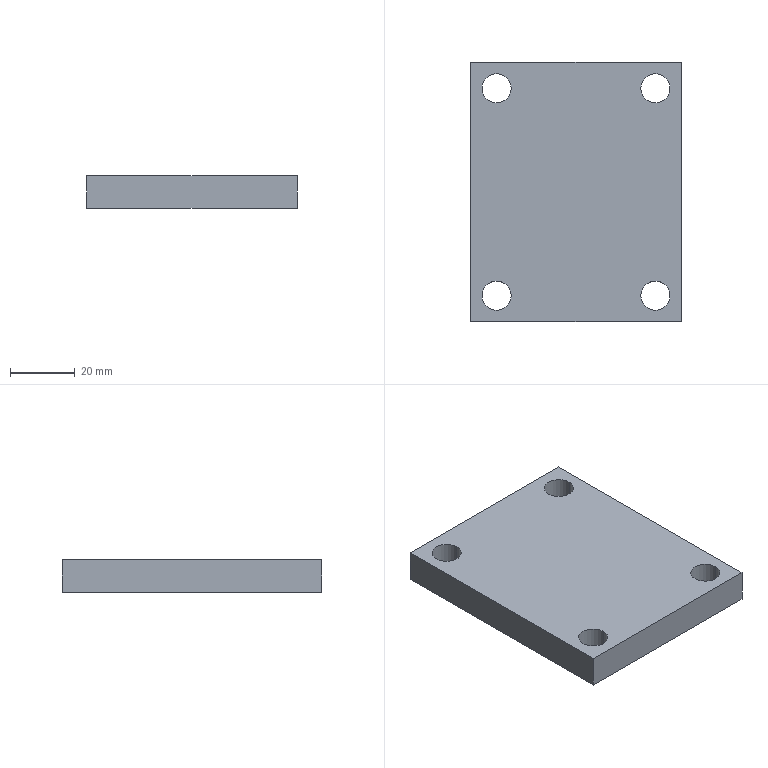Part | STEP file | X77-04206 | 1 solid | 14 faces | box 65 x 80 x 10 mm | volume 49455 mm3 | cylinder 8 | plane 6 | commonest cylinder face diameters 9 x8
STEP:
#1=CARTESIAN_POINT('',(18.828,-532.,10.));
#2=VERTEX_POINT('',#1);
#3=CARTESIAN_POINT('',(9.828,-532.,10.));
#4=VERTEX_POINT('',#3);
#5=CARTESIAN_POINT('',(14.328,-532.,10.));
#6=DIRECTION('',(0.,0.,-1.));
#7=DIRECTION('',(-1.,0.,0.));
#8=AXIS2_PLACEMENT_3D('',#5,#6,#7);
#9=CIRCLE('',#8,4.5);
#10=EDGE_CURVE('',#2,#4,#9,.T.);
#11=ORIENTED_EDGE('',*,*,#10,.F.);
#12=CARTESIAN_POINT('',(18.828,-532.,0.));
#13=VERTEX_POINT('',#12);
#14=CARTESIAN_POINT('',(18.828,-532.,10.));
#15=DIRECTION('',(0.,0.,-1.));
#16=VECTOR('',#15,1000.);
#17=LINE('',#14,#16);
#18=EDGE_CURVE('',#2,#13,#17,.T.);
#19=ORIENTED_EDGE('',*,*,#18,.T.);
#20=CARTESIAN_POINT('',(9.828,-532.,0.));
#21=VERTEX_POINT('',#20);
#22=CARTESIAN_POINT('',(14.328,-532.,0.));
#23=DIRECTION('',(0.,0.,-1.));
#24=DIRECTION('',(-1.,0.,0.));
#25=AXIS2_PLACEMENT_3D('',#22,#23,#24);
#26=CIRCLE('',#25,4.5);
#27=EDGE_CURVE('',#13,#21,#26,.T.);
#28=ORIENTED_EDGE('',*,*,#27,.T.);
#29=CARTESIAN_POINT('',(9.828,-532.,10.));
#30=DIRECTION('',(0.,0.,-1.));
#31=VECTOR('',#30,1000.);
#32=LINE('',#29,#31);
#33=EDGE_CURVE('',#4,#21,#32,.T.);
#34=ORIENTED_EDGE('',*,*,#33,.F.);
#35=EDGE_LOOP('',(#11,#19,#28,#34));
#36=FACE_OUTER_BOUND('',#35,.T.);
#37=CARTESIAN_POINT('',(14.328,-532.,10.));
#38=DIRECTION('',(0.,0.,-1.));
#39=DIRECTION('',(-1.,0.,0.));
#40=AXIS2_PLACEMENT_3D('',#37,#38,#39);
#41=CYLINDRICAL_SURFACE('',#40,4.5);
#42=ADVANCED_FACE('',(#36),#41,.F.);
#43=CARTESIAN_POINT('',(18.828,-468.,10.));
#44=VERTEX_POINT('',#43);
#45=CARTESIAN_POINT('',(9.828,-468.,10.));
#46=VERTEX_POINT('',#45);
#47=CARTESIAN_POINT('',(14.328,-468.,10.));
#48=DIRECTION('',(0.,0.,-1.));
#49=DIRECTION('',(-1.,0.,0.));
#50=AXIS2_PLACEMENT_3D('',#47,#48,#49);
#51=CIRCLE('',#50,4.5);
#52=EDGE_CURVE('',#44,#46,#51,.T.);
#53=ORIENTED_EDGE('',*,*,#52,.F.);
#54=CARTESIAN_POINT('',(18.828,-468.,0.));
#55=VERTEX_POINT('',#54);
#56=CARTESIAN_POINT('',(18.828,-468.,10.));
#57=DIRECTION('',(0.,0.,-1.));
#58=VECTOR('',#57,1000.);
#59=LINE('',#56,#58);
#60=EDGE_CURVE('',#44,#55,#59,.T.);
#61=ORIENTED_EDGE('',*,*,#60,.T.);
#62=CARTESIAN_POINT('',(9.828,-468.,0.));
#63=VERTEX_POINT('',#62);
#64=CARTESIAN_POINT('',(14.328,-468.,0.));
#65=DIRECTION('',(0.,0.,-1.));
#66=DIRECTION('',(-1.,0.,0.));
#67=AXIS2_PLACEMENT_3D('',#64,#65,#66);
#68=CIRCLE('',#67,4.5);
#69=EDGE_CURVE('',#55,#63,#68,.T.);
#70=ORIENTED_EDGE('',*,*,#69,.T.);
#71=CARTESIAN_POINT('',(9.828,-468.,10.));
#72=DIRECTION('',(0.,0.,-1.));
#73=VECTOR('',#72,1000.);
#74=LINE('',#71,#73);
#75=EDGE_CURVE('',#46,#63,#74,.T.);
#76=ORIENTED_EDGE('',*,*,#75,.F.);
#77=EDGE_LOOP('',(#53,#61,#70,#76));
#78=FACE_OUTER_BOUND('',#77,.T.);
#79=CARTESIAN_POINT('',(14.328,-468.,10.));
#80=DIRECTION('',(0.,0.,-1.));
#81=DIRECTION('',(-1.,0.,0.));
#82=AXIS2_PLACEMENT_3D('',#79,#80,#81);
#83=CYLINDRICAL_SURFACE('',#82,4.5);
#84=ADVANCED_FACE('',(#78),#83,.F.);
#85=CARTESIAN_POINT('',(-30.172,-468.,10.));
#86=VERTEX_POINT('',#85);
#87=CARTESIAN_POINT('',(-39.172,-468.,10.));
#88=VERTEX_POINT('',#87);
#89=CARTESIAN_POINT('',(-34.672,-468.,10.));
#90=DIRECTION('',(0.,0.,-1.));
#91=DIRECTION('',(-1.,0.,0.));
#92=AXIS2_PLACEMENT_3D('',#89,#90,#91);
#93=CIRCLE('',#92,4.5);
#94=EDGE_CURVE('',#86,#88,#93,.T.);
#95=ORIENTED_EDGE('',*,*,#94,.F.);
#96=CARTESIAN_POINT('',(-30.172,-468.,0.));
#97=VERTEX_POINT('',#96);
#98=CARTESIAN_POINT('',(-30.172,-468.,10.));
#99=DIRECTION('',(0.,0.,-1.));
#100=VECTOR('',#99,1000.);
#101=LINE('',#98,#100);
#102=EDGE_CURVE('',#86,#97,#101,.T.);
#103=ORIENTED_EDGE('',*,*,#102,.T.);
#104=CARTESIAN_POINT('',(-39.172,-468.,0.));
#105=VERTEX_POINT('',#104);
#106=CARTESIAN_POINT('',(-34.672,-468.,0.));
#107=DIRECTION('',(0.,0.,-1.));
#108=DIRECTION('',(-1.,0.,0.));
#109=AXIS2_PLACEMENT_3D('',#106,#107,#108);
#110=CIRCLE('',#109,4.5);
#111=EDGE_CURVE('',#97,#105,#110,.T.);
#112=ORIENTED_EDGE('',*,*,#111,.T.);
#113=CARTESIAN_POINT('',(-39.172,-468.,10.));
#114=DIRECTION('',(0.,0.,-1.));
#115=VECTOR('',#114,1000.);
#116=LINE('',#113,#115);
#117=EDGE_CURVE('',#88,#105,#116,.T.);
#118=ORIENTED_EDGE('',*,*,#117,.F.);
#119=EDGE_LOOP('',(#95,#103,#112,#118));
#120=FACE_OUTER_BOUND('',#119,.T.);
#121=CARTESIAN_POINT('',(-34.672,-468.,10.));
#122=DIRECTION('',(0.,0.,-1.));
#123=DIRECTION('',(-1.,0.,0.));
#124=AXIS2_PLACEMENT_3D('',#121,#122,#123);
#125=CYLINDRICAL_SURFACE('',#124,4.5);
#126=ADVANCED_FACE('',(#120),#125,.F.);
#127=CARTESIAN_POINT('',(-30.172,-532.,10.));
#128=VERTEX_POINT('',#127);
#129=CARTESIAN_POINT('',(-39.172,-532.,10.));
#130=VERTEX_POINT('',#129);
#131=CARTESIAN_POINT('',(-34.672,-532.,10.));
#132=DIRECTION('',(0.,0.,-1.));
#133=DIRECTION('',(-1.,0.,0.));
#134=AXIS2_PLACEMENT_3D('',#131,#132,#133);
#135=CIRCLE('',#134,4.5);
#136=EDGE_CURVE('',#128,#130,#135,.T.);
#137=ORIENTED_EDGE('',*,*,#136,.F.);
#138=CARTESIAN_POINT('',(-30.172,-532.,0.));
#139=VERTEX_POINT('',#138);
#140=CARTESIAN_POINT('',(-30.172,-532.,10.));
#141=DIRECTION('',(0.,0.,-1.));
#142=VECTOR('',#141,1000.);
#143=LINE('',#140,#142);
#144=EDGE_CURVE('',#128,#139,#143,.T.);
#145=ORIENTED_EDGE('',*,*,#144,.T.);
#146=CARTESIAN_POINT('',(-39.172,-532.,0.));
#147=VERTEX_POINT('',#146);
#148=CARTESIAN_POINT('',(-34.672,-532.,0.));
#149=DIRECTION('',(0.,0.,-1.));
#150=DIRECTION('',(-1.,0.,0.));
#151=AXIS2_PLACEMENT_3D('',#148,#149,#150);
#152=CIRCLE('',#151,4.5);
#153=EDGE_CURVE('',#139,#147,#152,.T.);
#154=ORIENTED_EDGE('',*,*,#153,.T.);
#155=CARTESIAN_POINT('',(-39.172,-532.,10.));
#156=DIRECTION('',(0.,0.,-1.));
#157=VECTOR('',#156,1000.);
#158=LINE('',#155,#157);
#159=EDGE_CURVE('',#130,#147,#158,.T.);
#160=ORIENTED_EDGE('',*,*,#159,.F.);
#161=EDGE_LOOP('',(#137,#145,#154,#160));
#162=FACE_OUTER_BOUND('',#161,.T.);
#163=CARTESIAN_POINT('',(-34.672,-532.,10.));
#164=DIRECTION('',(0.,0.,-1.));
#165=DIRECTION('',(-1.,0.,0.));
#166=AXIS2_PLACEMENT_3D('',#163,#164,#165);
#167=CYLINDRICAL_SURFACE('',#166,4.5);
#168=ADVANCED_FACE('',(#162),#167,.F.);
#169=CARTESIAN_POINT('',(22.328,-540.,0.));
#170=VERTEX_POINT('',#169);
#171=CARTESIAN_POINT('',(22.328,-460.,0.));
#172=VERTEX_POINT('',#171);
#173=CARTESIAN_POINT('',(22.328,-540.,0.));
#174=DIRECTION('',(0.,1.,0.));
#175=VECTOR('',#174,1000.);
#176=LINE('',#173,#175);
#177=EDGE_CURVE('',#170,#172,#176,.T.);
#178=ORIENTED_EDGE('',*,*,#177,.T.);
#179=CARTESIAN_POINT('',(22.328,-460.,10.));
#180=VERTEX_POINT('',#179);
#181=CARTESIAN_POINT('',(22.328,-460.,10.));
#182=DIRECTION('',(0.,0.,-1.));
#183=VECTOR('',#182,1000.);
#184=LINE('',#181,#183);
#185=EDGE_CURVE('',#180,#172,#184,.T.);
#186=ORIENTED_EDGE('',*,*,#185,.F.);
#187=CARTESIAN_POINT('',(22.328,-540.,10.));
#188=VERTEX_POINT('',#187);
#189=CARTESIAN_POINT('',(22.328,-540.,10.));
#190=DIRECTION('',(0.,1.,0.));
#191=VECTOR('',#190,1000.);
#192=LINE('',#189,#191);
#193=EDGE_CURVE('',#188,#180,#192,.T.);
#194=ORIENTED_EDGE('',*,*,#193,.F.);
#195=CARTESIAN_POINT('',(22.328,-540.,10.));
#196=DIRECTION('',(0.,0.,-1.));
#197=VECTOR('',#196,1000.);
#198=LINE('',#195,#197);
#199=EDGE_CURVE('',#188,#170,#198,.T.);
#200=ORIENTED_EDGE('',*,*,#199,.T.);
#201=EDGE_LOOP('',(#178,#186,#194,#200));
#202=FACE_OUTER_BOUND('',#201,.T.);
#203=CARTESIAN_POINT('',(22.328,-540.,10.));
#204=DIRECTION('',(-1.,0.,0.));
#205=DIRECTION('',(0.,0.,1.));
#206=AXIS2_PLACEMENT_3D('',#203,#204,#205);
#207=PLANE('',#206);
#208=ADVANCED_FACE('',(#202),#207,.F.);
#209=CARTESIAN_POINT('',(-42.672,-460.,0.));
#210=VERTEX_POINT('',#209);
#211=CARTESIAN_POINT('',(22.328,-460.,0.));
#212=DIRECTION('',(-1.,0.,0.));
#213=VECTOR('',#212,1000.);
#214=LINE('',#211,#213);
#215=EDGE_CURVE('',#172,#210,#214,.T.);
#216=ORIENTED_EDGE('',*,*,#215,.T.);
#217=CARTESIAN_POINT('',(-42.672,-460.,10.));
#218=VERTEX_POINT('',#217);
#219=CARTESIAN_POINT('',(-42.672,-460.,10.));
#220=DIRECTION('',(0.,0.,-1.));
#221=VECTOR('',#220,1000.);
#222=LINE('',#219,#221);
#223=EDGE_CURVE('',#218,#210,#222,.T.);
#224=ORIENTED_EDGE('',*,*,#223,.F.);
#225=CARTESIAN_POINT('',(22.328,-460.,10.));
#226=DIRECTION('',(-1.,0.,0.));
#227=VECTOR('',#226,1000.);
#228=LINE('',#225,#227);
#229=EDGE_CURVE('',#180,#218,#228,.T.);
#230=ORIENTED_EDGE('',*,*,#229,.F.);
#231=ORIENTED_EDGE('',*,*,#185,.T.);
#232=EDGE_LOOP('',(#216,#224,#230,#231));
#233=FACE_OUTER_BOUND('',#232,.T.);
#234=CARTESIAN_POINT('',(22.328,-460.,10.));
#235=DIRECTION('',(0.,-1.,0.));
#236=DIRECTION('',(0.,0.,-1.));
#237=AXIS2_PLACEMENT_3D('',#234,#235,#236);
#238=PLANE('',#237);
#239=ADVANCED_FACE('',(#233),#238,.F.);
#240=CARTESIAN_POINT('',(-42.672,-540.,0.));
#241=VERTEX_POINT('',#240);
#242=CARTESIAN_POINT('',(-42.672,-540.,0.));
#243=DIRECTION('',(0.,-1.,0.));
#244=VECTOR('',#243,1000.);
#245=LINE('',#242,#244);
#246=EDGE_CURVE('',#210,#241,#245,.T.);
#247=ORIENTED_EDGE('',*,*,#246,.T.);
#248=CARTESIAN_POINT('',(-42.672,-540.,10.));
#249=VERTEX_POINT('',#248);
#250=CARTESIAN_POINT('',(-42.672,-540.,10.));
#251=DIRECTION('',(0.,0.,-1.));
#252=VECTOR('',#251,1000.);
#253=LINE('',#250,#252);
#254=EDGE_CURVE('',#249,#241,#253,.T.);
#255=ORIENTED_EDGE('',*,*,#254,.F.);
#256=CARTESIAN_POINT('',(-42.672,-540.,10.));
#257=DIRECTION('',(0.,-1.,0.));
#258=VECTOR('',#257,1000.);
#259=LINE('',#256,#258);
#260=EDGE_CURVE('',#218,#249,#259,.T.);
#261=ORIENTED_EDGE('',*,*,#260,.F.);
#262=ORIENTED_EDGE('',*,*,#223,.T.);
#263=EDGE_LOOP('',(#247,#255,#261,#262));
#264=FACE_OUTER_BOUND('',#263,.T.);
#265=CARTESIAN_POINT('',(-42.672,-540.,10.));
#266=DIRECTION('',(1.,0.,0.));
#267=DIRECTION('',(0.,0.,-1.));
#268=AXIS2_PLACEMENT_3D('',#265,#266,#267);
#269=PLANE('',#268);
#270=ADVANCED_FACE('',(#264),#269,.F.);
#271=CARTESIAN_POINT('',(22.328,-540.,0.));
#272=DIRECTION('',(1.,0.,0.));
#273=VECTOR('',#272,1000.);
#274=LINE('',#271,#273);
#275=EDGE_CURVE('',#241,#170,#274,.T.);
#276=ORIENTED_EDGE('',*,*,#275,.T.);
#277=ORIENTED_EDGE('',*,*,#199,.F.);
#278=CARTESIAN_POINT('',(22.328,-540.,10.));
#279=DIRECTION('',(1.,0.,0.));
#280=VECTOR('',#279,1000.);
#281=LINE('',#278,#280);
#282=EDGE_CURVE('',#249,#188,#281,.T.);
#283=ORIENTED_EDGE('',*,*,#282,.F.);
#284=ORIENTED_EDGE('',*,*,#254,.T.);
#285=EDGE_LOOP('',(#276,#277,#283,#284));
#286=FACE_OUTER_BOUND('',#285,.T.);
#287=CARTESIAN_POINT('',(22.328,-540.,10.));
#288=DIRECTION('',(0.,1.,0.));
#289=DIRECTION('',(0.,0.,1.));
#290=AXIS2_PLACEMENT_3D('',#287,#288,#289);
#291=PLANE('',#290);
#292=ADVANCED_FACE('',(#286),#291,.F.);
#293=CARTESIAN_POINT('',(14.328,-532.,10.));
#294=DIRECTION('',(0.,0.,-1.));
#295=DIRECTION('',(-1.,0.,0.));
#296=AXIS2_PLACEMENT_3D('',#293,#294,#295);
#297=CIRCLE('',#296,4.5);
#298=EDGE_CURVE('',#4,#2,#297,.T.);
#299=ORIENTED_EDGE('',*,*,#298,.T.);
#300=ORIENTED_EDGE('',*,*,#10,.T.);
#301=EDGE_LOOP('',(#299,#300));
#302=FACE_BOUND('',#301,.T.);
#303=CARTESIAN_POINT('',(14.328,-468.,10.));
#304=DIRECTION('',(0.,0.,-1.));
#305=DIRECTION('',(-1.,0.,0.));
#306=AXIS2_PLACEMENT_3D('',#303,#304,#305);
#307=CIRCLE('',#306,4.5);
#308=EDGE_CURVE('',#46,#44,#307,.T.);
#309=ORIENTED_EDGE('',*,*,#308,.T.);
#310=ORIENTED_EDGE('',*,*,#52,.T.);
#311=EDGE_LOOP('',(#309,#310));
#312=FACE_BOUND('',#311,.T.);
#313=CARTESIAN_POINT('',(-34.672,-468.,10.));
#314=DIRECTION('',(0.,0.,-1.));
#315=DIRECTION('',(-1.,0.,0.));
#316=AXIS2_PLACEMENT_3D('',#313,#314,#315);
#317=CIRCLE('',#316,4.5);
#318=EDGE_CURVE('',#88,#86,#317,.T.);
#319=ORIENTED_EDGE('',*,*,#318,.T.);
#320=ORIENTED_EDGE('',*,*,#94,.T.);
#321=EDGE_LOOP('',(#319,#320));
#322=FACE_BOUND('',#321,.T.);
#323=CARTESIAN_POINT('',(-34.672,-532.,10.));
#324=DIRECTION('',(0.,0.,-1.));
#325=DIRECTION('',(-1.,0.,0.));
#326=AXIS2_PLACEMENT_3D('',#323,#324,#325);
#327=CIRCLE('',#326,4.5);
#328=EDGE_CURVE('',#130,#128,#327,.T.);
#329=ORIENTED_EDGE('',*,*,#328,.T.);
#330=ORIENTED_EDGE('',*,*,#136,.T.);
#331=EDGE_LOOP('',(#329,#330));
#332=FACE_BOUND('',#331,.T.);
#333=ORIENTED_EDGE('',*,*,#193,.T.);
#334=ORIENTED_EDGE('',*,*,#229,.T.);
#335=ORIENTED_EDGE('',*,*,#260,.T.);
#336=ORIENTED_EDGE('',*,*,#282,.T.);
#337=EDGE_LOOP('',(#333,#334,#335,#336));
#338=FACE_OUTER_BOUND('',#337,.T.);
#339=CARTESIAN_POINT('',(22.328,-460.,10.));
#340=DIRECTION('',(0.,0.,1.));
#341=DIRECTION('',(1.,0.,0.));
#342=AXIS2_PLACEMENT_3D('',#339,#340,#341);
#343=PLANE('',#342);
#344=ADVANCED_FACE('',(#302,#312,#322,#332,#338),#343,.T.);
#345=CARTESIAN_POINT('',(14.328,-532.,0.));
#346=DIRECTION('',(0.,0.,-1.));
#347=DIRECTION('',(-1.,0.,0.));
#348=AXIS2_PLACEMENT_3D('',#345,#346,#347);
#349=CIRCLE('',#348,4.5);
#350=EDGE_CURVE('',#21,#13,#349,.T.);
#351=ORIENTED_EDGE('',*,*,#350,.F.);
#352=ORIENTED_EDGE('',*,*,#27,.F.);
#353=EDGE_LOOP('',(#351,#352));
#354=FACE_BOUND('',#353,.T.);
#355=CARTESIAN_POINT('',(14.328,-468.,0.));
#356=DIRECTION('',(0.,0.,-1.));
#357=DIRECTION('',(-1.,0.,0.));
#358=AXIS2_PLACEMENT_3D('',#355,#356,#357);
#359=CIRCLE('',#358,4.5);
#360=EDGE_CURVE('',#63,#55,#359,.T.);
#361=ORIENTED_EDGE('',*,*,#360,.F.);
#362=ORIENTED_EDGE('',*,*,#69,.F.);
#363=EDGE_LOOP('',(#361,#362));
#364=FACE_BOUND('',#363,.T.);
#365=CARTESIAN_POINT('',(-34.672,-468.,0.));
#366=DIRECTION('',(0.,0.,-1.));
#367=DIRECTION('',(-1.,0.,0.));
#368=AXIS2_PLACEMENT_3D('',#365,#366,#367);
#369=CIRCLE('',#368,4.5);
#370=EDGE_CURVE('',#105,#97,#369,.T.);
#371=ORIENTED_EDGE('',*,*,#370,.F.);
#372=ORIENTED_EDGE('',*,*,#111,.F.);
#373=EDGE_LOOP('',(#371,#372));
#374=FACE_BOUND('',#373,.T.);
#375=CARTESIAN_POINT('',(-34.672,-532.,0.));
#376=DIRECTION('',(0.,0.,-1.));
#377=DIRECTION('',(-1.,0.,0.));
#378=AXIS2_PLACEMENT_3D('',#375,#376,#377);
#379=CIRCLE('',#378,4.5);
#380=EDGE_CURVE('',#147,#139,#379,.T.);
#381=ORIENTED_EDGE('',*,*,#380,.F.);
#382=ORIENTED_EDGE('',*,*,#153,.F.);
#383=EDGE_LOOP('',(#381,#382));
#384=FACE_BOUND('',#383,.T.);
#385=ORIENTED_EDGE('',*,*,#177,.F.);
#386=ORIENTED_EDGE('',*,*,#275,.F.);
#387=ORIENTED_EDGE('',*,*,#246,.F.);
#388=ORIENTED_EDGE('',*,*,#215,.F.);
#389=EDGE_LOOP('',(#385,#386,#387,#388));
#390=FACE_OUTER_BOUND('',#389,.T.);
#391=CARTESIAN_POINT('',(22.328,-460.,0.));
#392=DIRECTION('',(0.,0.,1.));
#393=DIRECTION('',(1.,0.,0.));
#394=AXIS2_PLACEMENT_3D('',#391,#392,#393);
#395=PLANE('',#394);
#396=ADVANCED_FACE('',(#354,#364,#374,#384,#390),#395,.F.);
#397=ORIENTED_EDGE('',*,*,#144,.F.);
#398=ORIENTED_EDGE('',*,*,#328,.F.);
#399=ORIENTED_EDGE('',*,*,#159,.T.);
#400=ORIENTED_EDGE('',*,*,#380,.T.);
#401=EDGE_LOOP('',(#397,#398,#399,#400));
#402=FACE_OUTER_BOUND('',#401,.T.);
#403=CARTESIAN_POINT('',(-34.672,-532.,10.));
#404=DIRECTION('',(0.,0.,-1.));
#405=DIRECTION('',(-1.,0.,0.));
#406=AXIS2_PLACEMENT_3D('',#403,#404,#405);
#407=CYLINDRICAL_SURFACE('',#406,4.5);
#408=ADVANCED_FACE('',(#402),#407,.F.);
#409=ORIENTED_EDGE('',*,*,#102,.F.);
#410=ORIENTED_EDGE('',*,*,#318,.F.);
#411=ORIENTED_EDGE('',*,*,#117,.T.);
#412=ORIENTED_EDGE('',*,*,#370,.T.);
#413=EDGE_LOOP('',(#409,#410,#411,#412));
#414=FACE_OUTER_BOUND('',#413,.T.);
#415=CARTESIAN_POINT('',(-34.672,-468.,10.));
#416=DIRECTION('',(0.,0.,-1.));
#417=DIRECTION('',(-1.,0.,0.));
#418=AXIS2_PLACEMENT_3D('',#415,#416,#417);
#419=CYLINDRICAL_SURFACE('',#418,4.5);
#420=ADVANCED_FACE('',(#414),#419,.F.);
#421=ORIENTED_EDGE('',*,*,#60,.F.);
#422=ORIENTED_EDGE('',*,*,#308,.F.);
#423=ORIENTED_EDGE('',*,*,#75,.T.);
#424=ORIENTED_EDGE('',*,*,#360,.T.);
#425=EDGE_LOOP('',(#421,#422,#423,#424));
#426=FACE_OUTER_BOUND('',#425,.T.);
#427=CARTESIAN_POINT('',(14.328,-468.,10.));
#428=DIRECTION('',(0.,0.,-1.));
#429=DIRECTION('',(-1.,0.,0.));
#430=AXIS2_PLACEMENT_3D('',#427,#428,#429);
#431=CYLINDRICAL_SURFACE('',#430,4.5);
#432=ADVANCED_FACE('',(#426),#431,.F.);
#433=ORIENTED_EDGE('',*,*,#18,.F.);
#434=ORIENTED_EDGE('',*,*,#298,.F.);
#435=ORIENTED_EDGE('',*,*,#33,.T.);
#436=ORIENTED_EDGE('',*,*,#350,.T.);
#437=EDGE_LOOP('',(#433,#434,#435,#436));
#438=FACE_OUTER_BOUND('',#437,.T.);
#439=CARTESIAN_POINT('',(14.328,-532.,10.));
#440=DIRECTION('',(0.,0.,-1.));
#441=DIRECTION('',(-1.,0.,0.));
#442=AXIS2_PLACEMENT_3D('',#439,#440,#441);
#443=CYLINDRICAL_SURFACE('',#442,4.5);
#444=ADVANCED_FACE('',(#438),#443,.F.);
#445=CLOSED_SHELL('',(#42,#84,#126,#168,#208,#239,#270,#292,#344,#396,#408,#420,#432,#444));
#446=MANIFOLD_SOLID_BREP('',#445);
#447=CARTESIAN_POINT('',(0.,0.,0.));
#448=DIRECTION('',(0.,0.,1.));
#449=DIRECTION('',(1.,0.,0.));
#450=AXIS2_PLACEMENT_3D('',#447,#448,#449);
#451=(LENGTH_UNIT()NAMED_UNIT(*)SI_UNIT(.MILLI.,.METRE.));
#452=UNCERTAINTY_MEASURE_WITH_UNIT(LENGTH_MEASURE(0.00001),#451,'','');
#453=(NAMED_UNIT(*)PLANE_ANGLE_UNIT()SI_UNIT($,.RADIAN.));
#454=(NAMED_UNIT(*)SI_UNIT($,.STERADIAN.)SOLID_ANGLE_UNIT());
#455=(GEOMETRIC_REPRESENTATION_CONTEXT(3)GLOBAL_UNCERTAINTY_ASSIGNED_CONTEXT((#452))GLOBAL_UNIT_ASSIGNED_CONTEXT((#451,#453,#454))REPRESENTATION_CONTEXT('',''));
#456=ADVANCED_BREP_SHAPE_REPRESENTATION('',(#446,#450),#455);